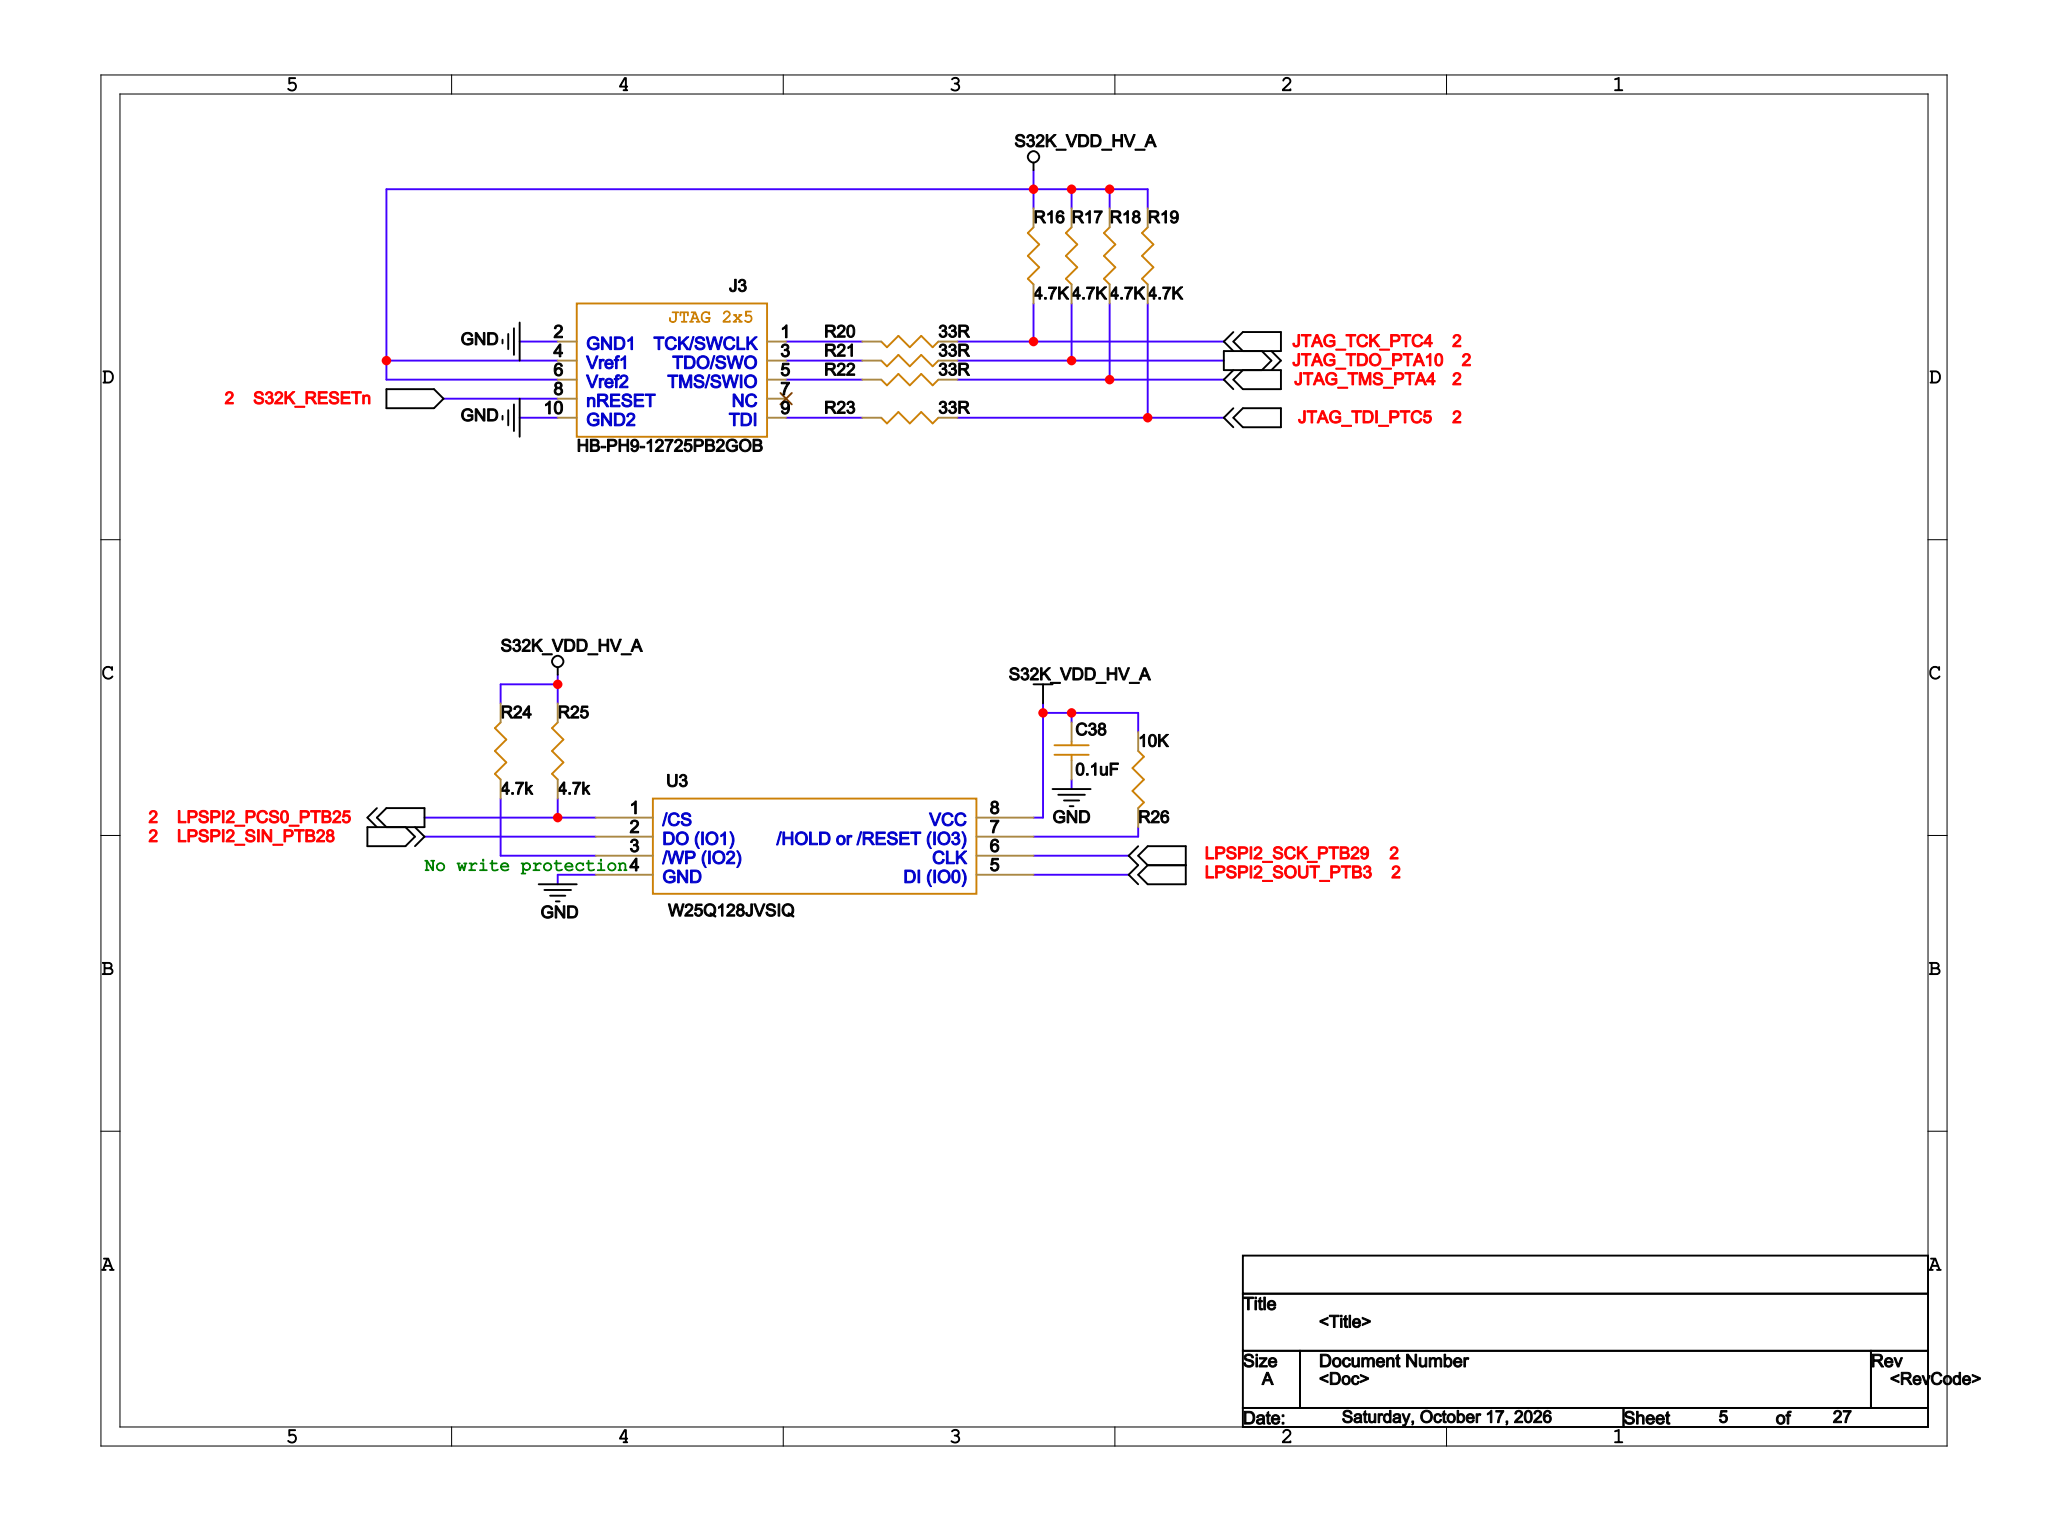Circuit board | Cadence Allegro | 477 parts | 327 nets | one sheet of the schematic
Parts on this sheet (reference | value | footprint):
C38 | 0.1uF | 0402
J3 | HB-PH9-12725PB2GOB | JTAG_2X5_1P27MM
R16 | 4.7K | 0402
R17 | 4.7K | 0402
R18 | 4.7K | 0402
R19 | 4.7K | 0402
R20 | 33R | 0402
R21 | 33R | 0402
R22 | 33R | 0402
R23 | 33R | 0402
R24 | 4.7K | 0402
R25 | 4.7K | 0402
R26 | 10K | 0402
U3 | W25Q128JVSIQ | SO8P_79_127_H220
Nets of these parts (net: part-pin ...):
N1674196: J3-1 R20-1
JTAG_TCK_PTC4: R16-1 R20-2
N1674242: J3-3 R21-1
JTAG_TDO_PTA10: R17-1 R21-2
N1674294: J3-5 R22-1
JTAG_TMS_PTA4: R18-1 R22-2
N1674346: J3-9 R23-1
JTAG_TDI_PTC5: R19-1 R23-2
GND: C38-2 J3-2 J3-10 U3-4
S32K_VDD_HV_A: C38-1 J3-4 J3-6 R16-2 R17-2 R18-2 R19-2 R24-1 R25-1 R26-2 U3-8
N2523682: R24-2 U3-3
LPSPI2_PCS0_PTB25: R25-2 U3-1
S32K_RESETN: J3-8
N1972160: R26-1 U3-7
LPSPI2_SIN_PTB28: U3-2
LPSPI2_SCK_PTB29: U3-6
LPSPI2_SOUT_PTB3: U3-5